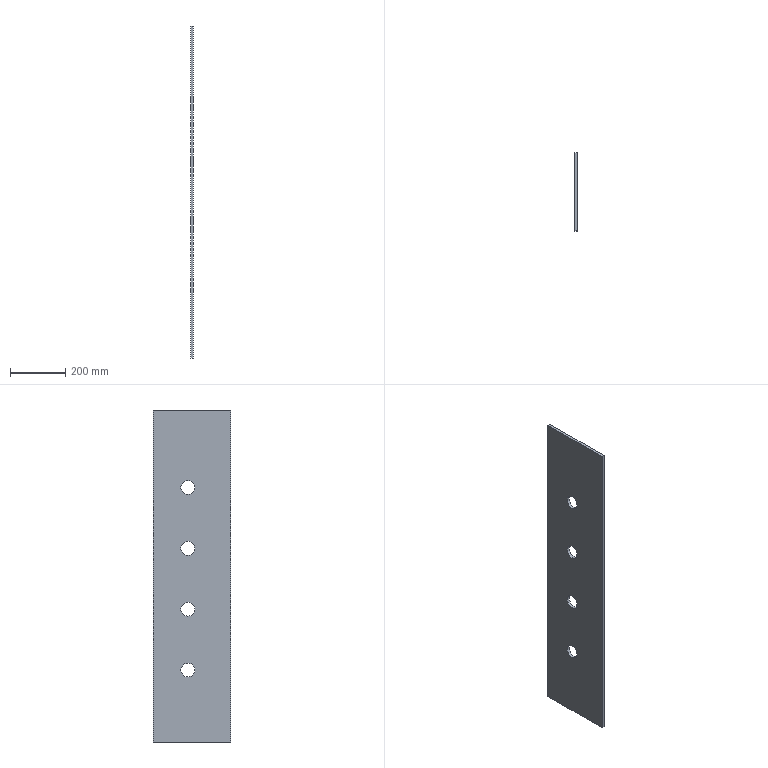Part | SolidWorks | features Extrusion 1, ICE 1, LPattern 1 | 1 solid | 14 faces | box 10 x 280 x 1200 mm | volume 3281460 mm3 | cylinder 8 | plane 6 | commonest cylinder face diameters 50 x8
STEP:
#1=CARTESIAN_POINT('',(0.,15.,125.));
#2=VERTEX_POINT('',#1);
#3=CARTESIAN_POINT('',(0.,15.,75.));
#4=VERTEX_POINT('',#3);
#5=CARTESIAN_POINT('',(0.,15.,100.));
#6=DIRECTION('',(1.,0.,0.));
#7=DIRECTION('',(0.,0.,-1.));
#8=AXIS2_PLACEMENT_3D('',#5,#6,#7);
#9=CIRCLE('',#8,25.);
#10=EDGE_CURVE('',#2,#4,#9,.T.);
#11=ORIENTED_EDGE('',*,*,#10,.F.);
#12=CARTESIAN_POINT('',(10.,15.,125.));
#13=VERTEX_POINT('',#12);
#14=CARTESIAN_POINT('',(0.,15.,125.));
#15=DIRECTION('',(1.,0.,0.));
#16=VECTOR('',#15,1000.);
#17=LINE('',#14,#16);
#18=EDGE_CURVE('',#2,#13,#17,.T.);
#19=ORIENTED_EDGE('',*,*,#18,.T.);
#20=CARTESIAN_POINT('',(10.,15.,75.));
#21=VERTEX_POINT('',#20);
#22=CARTESIAN_POINT('',(10.,15.,100.));
#23=DIRECTION('',(1.,0.,0.));
#24=DIRECTION('',(0.,0.,-1.));
#25=AXIS2_PLACEMENT_3D('',#22,#23,#24);
#26=CIRCLE('',#25,25.);
#27=EDGE_CURVE('',#13,#21,#26,.T.);
#28=ORIENTED_EDGE('',*,*,#27,.T.);
#29=CARTESIAN_POINT('',(0.,15.,75.));
#30=DIRECTION('',(1.,0.,0.));
#31=VECTOR('',#30,1000.);
#32=LINE('',#29,#31);
#33=EDGE_CURVE('',#4,#21,#32,.T.);
#34=ORIENTED_EDGE('',*,*,#33,.F.);
#35=EDGE_LOOP('',(#11,#19,#28,#34));
#36=FACE_OUTER_BOUND('',#35,.T.);
#37=CARTESIAN_POINT('',(0.,15.,100.));
#38=DIRECTION('',(1.,0.,0.));
#39=DIRECTION('',(0.,0.,-1.));
#40=AXIS2_PLACEMENT_3D('',#37,#38,#39);
#41=CYLINDRICAL_SURFACE('',#40,25.);
#42=ADVANCED_FACE('',(#36),#41,.F.);
#43=CARTESIAN_POINT('',(0.,15.,345.));
#44=VERTEX_POINT('',#43);
#45=CARTESIAN_POINT('',(0.,15.,295.));
#46=VERTEX_POINT('',#45);
#47=CARTESIAN_POINT('',(0.,15.,320.));
#48=DIRECTION('',(1.,0.,0.));
#49=DIRECTION('',(0.,0.,-1.));
#50=AXIS2_PLACEMENT_3D('',#47,#48,#49);
#51=CIRCLE('',#50,25.);
#52=EDGE_CURVE('',#44,#46,#51,.T.);
#53=ORIENTED_EDGE('',*,*,#52,.F.);
#54=CARTESIAN_POINT('',(10.,15.,345.));
#55=VERTEX_POINT('',#54);
#56=CARTESIAN_POINT('',(0.,15.,345.));
#57=DIRECTION('',(1.,0.,0.));
#58=VECTOR('',#57,1000.);
#59=LINE('',#56,#58);
#60=EDGE_CURVE('',#44,#55,#59,.T.);
#61=ORIENTED_EDGE('',*,*,#60,.T.);
#62=CARTESIAN_POINT('',(10.,15.,295.));
#63=VERTEX_POINT('',#62);
#64=CARTESIAN_POINT('',(10.,15.,320.));
#65=DIRECTION('',(1.,0.,0.));
#66=DIRECTION('',(0.,0.,-1.));
#67=AXIS2_PLACEMENT_3D('',#64,#65,#66);
#68=CIRCLE('',#67,25.);
#69=EDGE_CURVE('',#55,#63,#68,.T.);
#70=ORIENTED_EDGE('',*,*,#69,.T.);
#71=CARTESIAN_POINT('',(0.,15.,295.));
#72=DIRECTION('',(1.,0.,0.));
#73=VECTOR('',#72,1000.);
#74=LINE('',#71,#73);
#75=EDGE_CURVE('',#46,#63,#74,.T.);
#76=ORIENTED_EDGE('',*,*,#75,.F.);
#77=EDGE_LOOP('',(#53,#61,#70,#76));
#78=FACE_OUTER_BOUND('',#77,.T.);
#79=CARTESIAN_POINT('',(0.,15.,320.));
#80=DIRECTION('',(1.,0.,0.));
#81=DIRECTION('',(0.,0.,-1.));
#82=AXIS2_PLACEMENT_3D('',#79,#80,#81);
#83=CYLINDRICAL_SURFACE('',#82,25.);
#84=ADVANCED_FACE('',(#78),#83,.F.);
#85=CARTESIAN_POINT('',(0.,15.,-95.));
#86=VERTEX_POINT('',#85);
#87=CARTESIAN_POINT('',(0.,15.,-145.));
#88=VERTEX_POINT('',#87);
#89=CARTESIAN_POINT('',(0.,15.,-120.));
#90=DIRECTION('',(1.,0.,0.));
#91=DIRECTION('',(0.,0.,-1.));
#92=AXIS2_PLACEMENT_3D('',#89,#90,#91);
#93=CIRCLE('',#92,25.);
#94=EDGE_CURVE('',#86,#88,#93,.T.);
#95=ORIENTED_EDGE('',*,*,#94,.F.);
#96=CARTESIAN_POINT('',(10.,15.,-95.));
#97=VERTEX_POINT('',#96);
#98=CARTESIAN_POINT('',(0.,15.,-95.));
#99=DIRECTION('',(1.,0.,0.));
#100=VECTOR('',#99,1000.);
#101=LINE('',#98,#100);
#102=EDGE_CURVE('',#86,#97,#101,.T.);
#103=ORIENTED_EDGE('',*,*,#102,.T.);
#104=CARTESIAN_POINT('',(10.,15.,-145.));
#105=VERTEX_POINT('',#104);
#106=CARTESIAN_POINT('',(10.,15.,-120.));
#107=DIRECTION('',(1.,0.,0.));
#108=DIRECTION('',(0.,0.,-1.));
#109=AXIS2_PLACEMENT_3D('',#106,#107,#108);
#110=CIRCLE('',#109,25.);
#111=EDGE_CURVE('',#97,#105,#110,.T.);
#112=ORIENTED_EDGE('',*,*,#111,.T.);
#113=CARTESIAN_POINT('',(0.,15.,-145.));
#114=DIRECTION('',(1.,0.,0.));
#115=VECTOR('',#114,1000.);
#116=LINE('',#113,#115);
#117=EDGE_CURVE('',#88,#105,#116,.T.);
#118=ORIENTED_EDGE('',*,*,#117,.F.);
#119=EDGE_LOOP('',(#95,#103,#112,#118));
#120=FACE_OUTER_BOUND('',#119,.T.);
#121=CARTESIAN_POINT('',(0.,15.,-120.));
#122=DIRECTION('',(1.,0.,0.));
#123=DIRECTION('',(0.,0.,-1.));
#124=AXIS2_PLACEMENT_3D('',#121,#122,#123);
#125=CYLINDRICAL_SURFACE('',#124,25.);
#126=ADVANCED_FACE('',(#120),#125,.F.);
#127=CARTESIAN_POINT('',(0.,15.,-315.));
#128=VERTEX_POINT('',#127);
#129=CARTESIAN_POINT('',(0.,15.,-365.));
#130=VERTEX_POINT('',#129);
#131=CARTESIAN_POINT('',(0.,15.,-340.));
#132=DIRECTION('',(1.,0.,0.));
#133=DIRECTION('',(0.,0.,-1.));
#134=AXIS2_PLACEMENT_3D('',#131,#132,#133);
#135=CIRCLE('',#134,25.);
#136=EDGE_CURVE('',#128,#130,#135,.T.);
#137=ORIENTED_EDGE('',*,*,#136,.F.);
#138=CARTESIAN_POINT('',(10.,15.,-315.));
#139=VERTEX_POINT('',#138);
#140=CARTESIAN_POINT('',(0.,15.,-315.));
#141=DIRECTION('',(1.,0.,0.));
#142=VECTOR('',#141,1000.);
#143=LINE('',#140,#142);
#144=EDGE_CURVE('',#128,#139,#143,.T.);
#145=ORIENTED_EDGE('',*,*,#144,.T.);
#146=CARTESIAN_POINT('',(10.,15.,-365.));
#147=VERTEX_POINT('',#146);
#148=CARTESIAN_POINT('',(10.,15.,-340.));
#149=DIRECTION('',(1.,0.,0.));
#150=DIRECTION('',(0.,0.,-1.));
#151=AXIS2_PLACEMENT_3D('',#148,#149,#150);
#152=CIRCLE('',#151,25.);
#153=EDGE_CURVE('',#139,#147,#152,.T.);
#154=ORIENTED_EDGE('',*,*,#153,.T.);
#155=CARTESIAN_POINT('',(0.,15.,-365.));
#156=DIRECTION('',(1.,0.,0.));
#157=VECTOR('',#156,1000.);
#158=LINE('',#155,#157);
#159=EDGE_CURVE('',#130,#147,#158,.T.);
#160=ORIENTED_EDGE('',*,*,#159,.F.);
#161=EDGE_LOOP('',(#137,#145,#154,#160));
#162=FACE_OUTER_BOUND('',#161,.T.);
#163=CARTESIAN_POINT('',(0.,15.,-340.));
#164=DIRECTION('',(1.,0.,0.));
#165=DIRECTION('',(0.,0.,-1.));
#166=AXIS2_PLACEMENT_3D('',#163,#164,#165);
#167=CYLINDRICAL_SURFACE('',#166,25.);
#168=ADVANCED_FACE('',(#162),#167,.F.);
#169=ORIENTED_EDGE('',*,*,#144,.F.);
#170=CARTESIAN_POINT('',(0.,15.,-340.));
#171=DIRECTION('',(1.,0.,0.));
#172=DIRECTION('',(0.,0.,-1.));
#173=AXIS2_PLACEMENT_3D('',#170,#171,#172);
#174=CIRCLE('',#173,25.);
#175=EDGE_CURVE('',#130,#128,#174,.T.);
#176=ORIENTED_EDGE('',*,*,#175,.F.);
#177=ORIENTED_EDGE('',*,*,#159,.T.);
#178=CARTESIAN_POINT('',(10.,15.,-340.));
#179=DIRECTION('',(1.,0.,0.));
#180=DIRECTION('',(0.,0.,-1.));
#181=AXIS2_PLACEMENT_3D('',#178,#179,#180);
#182=CIRCLE('',#181,25.);
#183=EDGE_CURVE('',#147,#139,#182,.T.);
#184=ORIENTED_EDGE('',*,*,#183,.T.);
#185=EDGE_LOOP('',(#169,#176,#177,#184));
#186=FACE_OUTER_BOUND('',#185,.T.);
#187=CARTESIAN_POINT('',(0.,15.,-340.));
#188=DIRECTION('',(1.,0.,0.));
#189=DIRECTION('',(0.,0.,-1.));
#190=AXIS2_PLACEMENT_3D('',#187,#188,#189);
#191=CYLINDRICAL_SURFACE('',#190,25.);
#192=ADVANCED_FACE('',(#186),#191,.F.);
#193=ORIENTED_EDGE('',*,*,#102,.F.);
#194=CARTESIAN_POINT('',(0.,15.,-120.));
#195=DIRECTION('',(1.,0.,0.));
#196=DIRECTION('',(0.,0.,-1.));
#197=AXIS2_PLACEMENT_3D('',#194,#195,#196);
#198=CIRCLE('',#197,25.);
#199=EDGE_CURVE('',#88,#86,#198,.T.);
#200=ORIENTED_EDGE('',*,*,#199,.F.);
#201=ORIENTED_EDGE('',*,*,#117,.T.);
#202=CARTESIAN_POINT('',(10.,15.,-120.));
#203=DIRECTION('',(1.,0.,0.));
#204=DIRECTION('',(0.,0.,-1.));
#205=AXIS2_PLACEMENT_3D('',#202,#203,#204);
#206=CIRCLE('',#205,25.);
#207=EDGE_CURVE('',#105,#97,#206,.T.);
#208=ORIENTED_EDGE('',*,*,#207,.T.);
#209=EDGE_LOOP('',(#193,#200,#201,#208));
#210=FACE_OUTER_BOUND('',#209,.T.);
#211=CARTESIAN_POINT('',(0.,15.,-120.));
#212=DIRECTION('',(1.,0.,0.));
#213=DIRECTION('',(0.,0.,-1.));
#214=AXIS2_PLACEMENT_3D('',#211,#212,#213);
#215=CYLINDRICAL_SURFACE('',#214,25.);
#216=ADVANCED_FACE('',(#210),#215,.F.);
#217=CARTESIAN_POINT('',(0.,-140.,-600.));
#218=VERTEX_POINT('',#217);
#219=CARTESIAN_POINT('',(0.,140.,-600.));
#220=VERTEX_POINT('',#219);
#221=CARTESIAN_POINT('',(0.,-140.,-600.));
#222=DIRECTION('',(0.,1.,0.));
#223=VECTOR('',#222,1000.);
#224=LINE('',#221,#223);
#225=EDGE_CURVE('',#218,#220,#224,.T.);
#226=ORIENTED_EDGE('',*,*,#225,.T.);
#227=CARTESIAN_POINT('',(10.,140.,-600.));
#228=VERTEX_POINT('',#227);
#229=CARTESIAN_POINT('',(10.,140.,-600.));
#230=DIRECTION('',(-1.,0.,0.));
#231=VECTOR('',#230,1000.);
#232=LINE('',#229,#231);
#233=EDGE_CURVE('',#228,#220,#232,.T.);
#234=ORIENTED_EDGE('',*,*,#233,.F.);
#235=CARTESIAN_POINT('',(10.,-140.,-600.));
#236=VERTEX_POINT('',#235);
#237=CARTESIAN_POINT('',(10.,-140.,-600.));
#238=DIRECTION('',(0.,1.,0.));
#239=VECTOR('',#238,1000.);
#240=LINE('',#237,#239);
#241=EDGE_CURVE('',#236,#228,#240,.T.);
#242=ORIENTED_EDGE('',*,*,#241,.F.);
#243=CARTESIAN_POINT('',(10.,-140.,-600.));
#244=DIRECTION('',(-1.,0.,0.));
#245=VECTOR('',#244,1000.);
#246=LINE('',#243,#245);
#247=EDGE_CURVE('',#236,#218,#246,.T.);
#248=ORIENTED_EDGE('',*,*,#247,.T.);
#249=EDGE_LOOP('',(#226,#234,#242,#248));
#250=FACE_OUTER_BOUND('',#249,.T.);
#251=CARTESIAN_POINT('',(10.,-140.,-600.));
#252=DIRECTION('',(0.,0.,1.));
#253=DIRECTION('',(1.,0.,0.));
#254=AXIS2_PLACEMENT_3D('',#251,#252,#253);
#255=PLANE('',#254);
#256=ADVANCED_FACE('',(#250),#255,.F.);
#257=CARTESIAN_POINT('',(0.,140.,600.));
#258=VERTEX_POINT('',#257);
#259=CARTESIAN_POINT('',(0.,140.,600.));
#260=DIRECTION('',(0.,0.,1.));
#261=VECTOR('',#260,1000.);
#262=LINE('',#259,#261);
#263=EDGE_CURVE('',#220,#258,#262,.T.);
#264=ORIENTED_EDGE('',*,*,#263,.T.);
#265=CARTESIAN_POINT('',(10.,140.,600.));
#266=VERTEX_POINT('',#265);
#267=CARTESIAN_POINT('',(10.,140.,600.));
#268=DIRECTION('',(-1.,0.,0.));
#269=VECTOR('',#268,1000.);
#270=LINE('',#267,#269);
#271=EDGE_CURVE('',#266,#258,#270,.T.);
#272=ORIENTED_EDGE('',*,*,#271,.F.);
#273=CARTESIAN_POINT('',(10.,140.,600.));
#274=DIRECTION('',(0.,0.,1.));
#275=VECTOR('',#274,1000.);
#276=LINE('',#273,#275);
#277=EDGE_CURVE('',#228,#266,#276,.T.);
#278=ORIENTED_EDGE('',*,*,#277,.F.);
#279=ORIENTED_EDGE('',*,*,#233,.T.);
#280=EDGE_LOOP('',(#264,#272,#278,#279));
#281=FACE_OUTER_BOUND('',#280,.T.);
#282=CARTESIAN_POINT('',(10.,140.,600.));
#283=DIRECTION('',(0.,-1.,0.));
#284=DIRECTION('',(0.,0.,-1.));
#285=AXIS2_PLACEMENT_3D('',#282,#283,#284);
#286=PLANE('',#285);
#287=ADVANCED_FACE('',(#281),#286,.F.);
#288=CARTESIAN_POINT('',(0.,-140.,600.));
#289=VERTEX_POINT('',#288);
#290=CARTESIAN_POINT('',(0.,-140.,600.));
#291=DIRECTION('',(0.,-1.,0.));
#292=VECTOR('',#291,1000.);
#293=LINE('',#290,#292);
#294=EDGE_CURVE('',#258,#289,#293,.T.);
#295=ORIENTED_EDGE('',*,*,#294,.T.);
#296=CARTESIAN_POINT('',(10.,-140.,600.));
#297=VERTEX_POINT('',#296);
#298=CARTESIAN_POINT('',(10.,-140.,600.));
#299=DIRECTION('',(-1.,0.,0.));
#300=VECTOR('',#299,1000.);
#301=LINE('',#298,#300);
#302=EDGE_CURVE('',#297,#289,#301,.T.);
#303=ORIENTED_EDGE('',*,*,#302,.F.);
#304=CARTESIAN_POINT('',(10.,-140.,600.));
#305=DIRECTION('',(0.,-1.,0.));
#306=VECTOR('',#305,1000.);
#307=LINE('',#304,#306);
#308=EDGE_CURVE('',#266,#297,#307,.T.);
#309=ORIENTED_EDGE('',*,*,#308,.F.);
#310=ORIENTED_EDGE('',*,*,#271,.T.);
#311=EDGE_LOOP('',(#295,#303,#309,#310));
#312=FACE_OUTER_BOUND('',#311,.T.);
#313=CARTESIAN_POINT('',(10.,-140.,600.));
#314=DIRECTION('',(0.,0.,-1.));
#315=DIRECTION('',(-1.,0.,0.));
#316=AXIS2_PLACEMENT_3D('',#313,#314,#315);
#317=PLANE('',#316);
#318=ADVANCED_FACE('',(#312),#317,.F.);
#319=CARTESIAN_POINT('',(0.,-140.,600.));
#320=DIRECTION('',(0.,0.,-1.));
#321=VECTOR('',#320,1000.);
#322=LINE('',#319,#321);
#323=EDGE_CURVE('',#289,#218,#322,.T.);
#324=ORIENTED_EDGE('',*,*,#323,.T.);
#325=ORIENTED_EDGE('',*,*,#247,.F.);
#326=CARTESIAN_POINT('',(10.,-140.,600.));
#327=DIRECTION('',(0.,0.,-1.));
#328=VECTOR('',#327,1000.);
#329=LINE('',#326,#328);
#330=EDGE_CURVE('',#297,#236,#329,.T.);
#331=ORIENTED_EDGE('',*,*,#330,.F.);
#332=ORIENTED_EDGE('',*,*,#302,.T.);
#333=EDGE_LOOP('',(#324,#325,#331,#332));
#334=FACE_OUTER_BOUND('',#333,.T.);
#335=CARTESIAN_POINT('',(10.,-140.,600.));
#336=DIRECTION('',(0.,1.,0.));
#337=DIRECTION('',(0.,0.,1.));
#338=AXIS2_PLACEMENT_3D('',#335,#336,#337);
#339=PLANE('',#338);
#340=ADVANCED_FACE('',(#334),#339,.F.);
#341=CARTESIAN_POINT('',(10.,15.,100.));
#342=DIRECTION('',(1.,0.,0.));
#343=DIRECTION('',(0.,0.,-1.));
#344=AXIS2_PLACEMENT_3D('',#341,#342,#343);
#345=CIRCLE('',#344,25.);
#346=EDGE_CURVE('',#21,#13,#345,.T.);
#347=ORIENTED_EDGE('',*,*,#346,.F.);
#348=ORIENTED_EDGE('',*,*,#27,.F.);
#349=EDGE_LOOP('',(#347,#348));
#350=FACE_BOUND('',#349,.T.);
#351=CARTESIAN_POINT('',(10.,15.,320.));
#352=DIRECTION('',(1.,0.,0.));
#353=DIRECTION('',(0.,0.,-1.));
#354=AXIS2_PLACEMENT_3D('',#351,#352,#353);
#355=CIRCLE('',#354,25.);
#356=EDGE_CURVE('',#63,#55,#355,.T.);
#357=ORIENTED_EDGE('',*,*,#356,.F.);
#358=ORIENTED_EDGE('',*,*,#69,.F.);
#359=EDGE_LOOP('',(#357,#358));
#360=FACE_BOUND('',#359,.T.);
#361=ORIENTED_EDGE('',*,*,#241,.T.);
#362=ORIENTED_EDGE('',*,*,#277,.T.);
#363=ORIENTED_EDGE('',*,*,#308,.T.);
#364=ORIENTED_EDGE('',*,*,#330,.T.);
#365=EDGE_LOOP('',(#361,#362,#363,#364));
#366=FACE_OUTER_BOUND('',#365,.T.);
#367=ORIENTED_EDGE('',*,*,#207,.F.);
#368=ORIENTED_EDGE('',*,*,#111,.F.);
#369=EDGE_LOOP('',(#367,#368));
#370=FACE_BOUND('',#369,.T.);
#371=ORIENTED_EDGE('',*,*,#183,.F.);
#372=ORIENTED_EDGE('',*,*,#153,.F.);
#373=EDGE_LOOP('',(#371,#372));
#374=FACE_BOUND('',#373,.T.);
#375=CARTESIAN_POINT('',(10.,0.,0.));
#376=DIRECTION('',(-1.,0.,0.));
#377=DIRECTION('',(0.,0.,1.));
#378=AXIS2_PLACEMENT_3D('',#375,#376,#377);
#379=PLANE('',#378);
#380=ADVANCED_FACE('',(#350,#360,#366,#370,#374),#379,.F.);
#381=CARTESIAN_POINT('',(0.,15.,100.));
#382=DIRECTION('',(1.,0.,0.));
#383=DIRECTION('',(0.,0.,-1.));
#384=AXIS2_PLACEMENT_3D('',#381,#382,#383);
#385=CIRCLE('',#384,25.);
#386=EDGE_CURVE('',#4,#2,#385,.T.);
#387=ORIENTED_EDGE('',*,*,#386,.T.);
#388=ORIENTED_EDGE('',*,*,#10,.T.);
#389=EDGE_LOOP('',(#387,#388));
#390=FACE_BOUND('',#389,.T.);
#391=CARTESIAN_POINT('',(0.,15.,320.));
#392=DIRECTION('',(1.,0.,0.));
#393=DIRECTION('',(0.,0.,-1.));
#394=AXIS2_PLACEMENT_3D('',#391,#392,#393);
#395=CIRCLE('',#394,25.);
#396=EDGE_CURVE('',#46,#44,#395,.T.);
#397=ORIENTED_EDGE('',*,*,#396,.T.);
#398=ORIENTED_EDGE('',*,*,#52,.T.);
#399=EDGE_LOOP('',(#397,#398));
#400=FACE_BOUND('',#399,.T.);
#401=ORIENTED_EDGE('',*,*,#225,.F.);
#402=ORIENTED_EDGE('',*,*,#323,.F.);
#403=ORIENTED_EDGE('',*,*,#294,.F.);
#404=ORIENTED_EDGE('',*,*,#263,.F.);
#405=EDGE_LOOP('',(#401,#402,#403,#404));
#406=FACE_OUTER_BOUND('',#405,.T.);
#407=ORIENTED_EDGE('',*,*,#199,.T.);
#408=ORIENTED_EDGE('',*,*,#94,.T.);
#409=EDGE_LOOP('',(#407,#408));
#410=FACE_BOUND('',#409,.T.);
#411=ORIENTED_EDGE('',*,*,#175,.T.);
#412=ORIENTED_EDGE('',*,*,#136,.T.);
#413=EDGE_LOOP('',(#411,#412));
#414=FACE_BOUND('',#413,.T.);
#415=CARTESIAN_POINT('',(0.,0.,0.));
#416=DIRECTION('',(-1.,0.,0.));
#417=DIRECTION('',(0.,0.,1.));
#418=AXIS2_PLACEMENT_3D('',#415,#416,#417);
#419=PLANE('',#418);
#420=ADVANCED_FACE('',(#390,#400,#406,#410,#414),#419,.T.);
#421=ORIENTED_EDGE('',*,*,#60,.F.);
#422=ORIENTED_EDGE('',*,*,#396,.F.);
#423=ORIENTED_EDGE('',*,*,#75,.T.);
#424=ORIENTED_EDGE('',*,*,#356,.T.);
#425=EDGE_LOOP('',(#421,#422,#423,#424));
#426=FACE_OUTER_BOUND('',#425,.T.);
#427=CARTESIAN_POINT('',(0.,15.,320.));
#428=DIRECTION('',(1.,0.,0.));
#429=DIRECTION('',(0.,0.,-1.));
#430=AXIS2_PLACEMENT_3D('',#427,#428,#429);
#431=CYLINDRICAL_SURFACE('',#430,25.);
#432=ADVANCED_FACE('',(#426),#431,.F.);
#433=ORIENTED_EDGE('',*,*,#18,.F.);
#434=ORIENTED_EDGE('',*,*,#386,.F.);
#435=ORIENTED_EDGE('',*,*,#33,.T.);
#436=ORIENTED_EDGE('',*,*,#346,.T.);
#437=EDGE_LOOP('',(#433,#434,#435,#436));
#438=FACE_OUTER_BOUND('',#437,.T.);
#439=CARTESIAN_POINT('',(0.,15.,100.));
#440=DIRECTION('',(1.,0.,0.));
#441=DIRECTION('',(0.,0.,-1.));
#442=AXIS2_PLACEMENT_3D('',#439,#440,#441);
#443=CYLINDRICAL_SURFACE('',#442,25.);
#444=ADVANCED_FACE('',(#438),#443,.F.);
#445=CLOSED_SHELL('',(#42,#84,#126,#168,#192,#216,#256,#287,#318,#340,#380,#420,#432,#444));
#446=MANIFOLD_SOLID_BREP('',#445);
#447=CARTESIAN_POINT('',(0.,0.,0.));
#448=DIRECTION('',(0.,0.,1.));
#449=DIRECTION('',(1.,0.,0.));
#450=AXIS2_PLACEMENT_3D('',#447,#448,#449);
#451=(LENGTH_UNIT()NAMED_UNIT(*)SI_UNIT(.MILLI.,.METRE.));
#452=UNCERTAINTY_MEASURE_WITH_UNIT(LENGTH_MEASURE(0.00001),#451,'','');
#453=(NAMED_UNIT(*)PLANE_ANGLE_UNIT()SI_UNIT($,.RADIAN.));
#454=(NAMED_UNIT(*)SI_UNIT($,.STERADIAN.)SOLID_ANGLE_UNIT());
#455=(GEOMETRIC_REPRESENTATION_CONTEXT(3)GLOBAL_UNCERTAINTY_ASSIGNED_CONTEXT((#452))GLOBAL_UNIT_ASSIGNED_CONTEXT((#451,#453,#454))REPRESENTATION_CONTEXT('',''));
#456=ADVANCED_BREP_SHAPE_REPRESENTATION('',(#446,#450),#455);